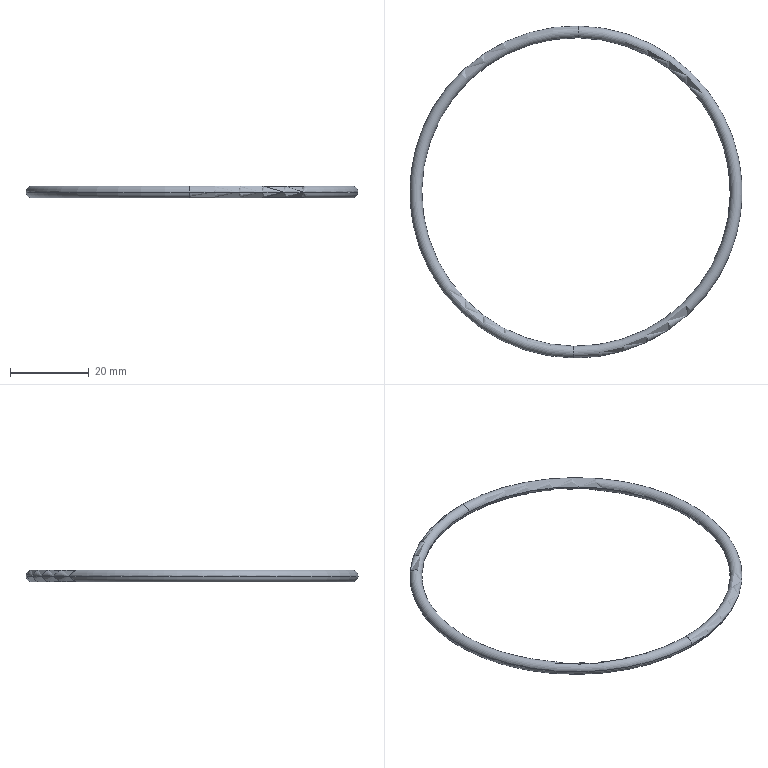Part | SolidWorks | features BaseBody 1 | 1 solid | 4 faces | box 84.4 x 84.4 x 3 mm | volume 1808 mm3 | torus 4
STEP:
#1=CARTESIAN_POINT('',(-43.838,-7.908,87.25));
#2=VERTEX_POINT('',#1);
#3=CARTESIAN_POINT('',(-43.882,-10.908,87.25));
#4=VERTEX_POINT('',#3);
#5=CARTESIAN_POINT('',(-43.86,-9.408,87.25));
#6=DIRECTION('',(-0.9999,0.01482,0.));
#7=DIRECTION('',(-0.01482,-0.9999,0.));
#8=AXIS2_PLACEMENT_3D('',#5,#6,#7);
#9=CIRCLE('',#8,1.5);
#10=EDGE_CURVE('',#2,#4,#9,.T.);
#11=ORIENTED_EDGE('',*,*,#10,.F.);
#12=CARTESIAN_POINT('',(-45.088,-92.299,87.25));
#13=VERTEX_POINT('',#12);
#14=CARTESIAN_POINT('',(-44.463,-50.104,87.25));
#15=DIRECTION('',(0.,0.,-1.));
#16=DIRECTION('',(-1.,0.,0.));
#17=AXIS2_PLACEMENT_3D('',#14,#15,#16);
#18=CIRCLE('',#17,42.2);
#19=EDGE_CURVE('',#2,#13,#18,.T.);
#20=ORIENTED_EDGE('',*,*,#19,.T.);
#21=CARTESIAN_POINT('',(-45.044,-89.299,87.25));
#22=VERTEX_POINT('',#21);
#23=CARTESIAN_POINT('',(-45.066,-90.799,87.25));
#24=DIRECTION('',(0.9999,-0.01482,0.));
#25=DIRECTION('',(0.01482,0.9999,0.));
#26=AXIS2_PLACEMENT_3D('',#23,#24,#25);
#27=CIRCLE('',#26,1.5);
#28=EDGE_CURVE('',#13,#22,#27,.T.);
#29=ORIENTED_EDGE('',*,*,#28,.T.);
#30=CARTESIAN_POINT('',(-44.463,-50.104,87.25));
#31=DIRECTION('',(0.,0.,-1.));
#32=DIRECTION('',(-1.,0.,0.));
#33=AXIS2_PLACEMENT_3D('',#30,#31,#32);
#34=CIRCLE('',#33,39.2);
#35=EDGE_CURVE('',#4,#22,#34,.T.);
#36=ORIENTED_EDGE('',*,*,#35,.F.);
#37=EDGE_LOOP('',(#11,#20,#29,#36));
#38=FACE_OUTER_BOUND('',#37,.T.);
#39=CARTESIAN_POINT('',(-44.463,-50.104,87.25));
#40=DIRECTION('',(0.,0.,-1.));
#41=DIRECTION('',(-0.01482,-0.9999,0.));
#42=AXIS2_PLACEMENT_3D('',#39,#40,#41);
#43=TOROIDAL_SURFACE('',#42,40.7,1.5);
#44=ADVANCED_FACE('',(#38),#43,.T.);
#45=ORIENTED_EDGE('',*,*,#28,.F.);
#46=CARTESIAN_POINT('',(-44.463,-50.104,87.25));
#47=DIRECTION('',(0.,0.,-1.));
#48=DIRECTION('',(-1.,0.,0.));
#49=AXIS2_PLACEMENT_3D('',#46,#47,#48);
#50=CIRCLE('',#49,42.2);
#51=EDGE_CURVE('',#13,#2,#50,.T.);
#52=ORIENTED_EDGE('',*,*,#51,.T.);
#53=ORIENTED_EDGE('',*,*,#10,.T.);
#54=CARTESIAN_POINT('',(-44.463,-50.104,87.25));
#55=DIRECTION('',(0.,0.,-1.));
#56=DIRECTION('',(-1.,0.,0.));
#57=AXIS2_PLACEMENT_3D('',#54,#55,#56);
#58=CIRCLE('',#57,39.2);
#59=EDGE_CURVE('',#22,#4,#58,.T.);
#60=ORIENTED_EDGE('',*,*,#59,.F.);
#61=EDGE_LOOP('',(#45,#52,#53,#60));
#62=FACE_OUTER_BOUND('',#61,.T.);
#63=CARTESIAN_POINT('',(-44.463,-50.104,87.25));
#64=DIRECTION('',(0.,0.,-1.));
#65=DIRECTION('',(-0.01482,-0.9999,0.));
#66=AXIS2_PLACEMENT_3D('',#63,#64,#65);
#67=TOROIDAL_SURFACE('',#66,40.7,1.5);
#68=ADVANCED_FACE('',(#62),#67,.T.);
#69=ORIENTED_EDGE('',*,*,#51,.F.);
#70=CARTESIAN_POINT('',(-45.066,-90.799,87.25));
#71=DIRECTION('',(0.9999,-0.01482,0.));
#72=DIRECTION('',(0.01482,0.9999,0.));
#73=AXIS2_PLACEMENT_3D('',#70,#71,#72);
#74=CIRCLE('',#73,1.5);
#75=EDGE_CURVE('',#22,#13,#74,.T.);
#76=ORIENTED_EDGE('',*,*,#75,.F.);
#77=ORIENTED_EDGE('',*,*,#59,.T.);
#78=CARTESIAN_POINT('',(-43.86,-9.408,87.25));
#79=DIRECTION('',(-0.9999,0.01482,0.));
#80=DIRECTION('',(-0.01482,-0.9999,0.));
#81=AXIS2_PLACEMENT_3D('',#78,#79,#80);
#82=CIRCLE('',#81,1.5);
#83=EDGE_CURVE('',#4,#2,#82,.T.);
#84=ORIENTED_EDGE('',*,*,#83,.T.);
#85=EDGE_LOOP('',(#69,#76,#77,#84));
#86=FACE_OUTER_BOUND('',#85,.T.);
#87=CARTESIAN_POINT('',(-44.463,-50.104,87.25));
#88=DIRECTION('',(0.,0.,-1.));
#89=DIRECTION('',(-0.01482,-0.9999,0.));
#90=AXIS2_PLACEMENT_3D('',#87,#88,#89);
#91=TOROIDAL_SURFACE('',#90,40.7,1.5);
#92=ADVANCED_FACE('',(#86),#91,.T.);
#93=ORIENTED_EDGE('',*,*,#19,.F.);
#94=ORIENTED_EDGE('',*,*,#83,.F.);
#95=ORIENTED_EDGE('',*,*,#35,.T.);
#96=ORIENTED_EDGE('',*,*,#75,.T.);
#97=EDGE_LOOP('',(#93,#94,#95,#96));
#98=FACE_OUTER_BOUND('',#97,.T.);
#99=CARTESIAN_POINT('',(-44.463,-50.104,87.25));
#100=DIRECTION('',(0.,0.,-1.));
#101=DIRECTION('',(-0.01482,-0.9999,0.));
#102=AXIS2_PLACEMENT_3D('',#99,#100,#101);
#103=TOROIDAL_SURFACE('',#102,40.7,1.5);
#104=ADVANCED_FACE('',(#98),#103,.T.);
#105=CLOSED_SHELL('',(#44,#68,#92,#104));
#106=MANIFOLD_SOLID_BREP('',#105);
#107=CARTESIAN_POINT('',(0.,0.,0.));
#108=DIRECTION('',(0.,0.,1.));
#109=DIRECTION('',(1.,0.,0.));
#110=AXIS2_PLACEMENT_3D('',#107,#108,#109);
#111=(LENGTH_UNIT()NAMED_UNIT(*)SI_UNIT(.MILLI.,.METRE.));
#112=UNCERTAINTY_MEASURE_WITH_UNIT(LENGTH_MEASURE(0.00001),#111,'','');
#113=(NAMED_UNIT(*)PLANE_ANGLE_UNIT()SI_UNIT($,.RADIAN.));
#114=(NAMED_UNIT(*)SI_UNIT($,.STERADIAN.)SOLID_ANGLE_UNIT());
#115=(GEOMETRIC_REPRESENTATION_CONTEXT(3)GLOBAL_UNCERTAINTY_ASSIGNED_CONTEXT((#112))GLOBAL_UNIT_ASSIGNED_CONTEXT((#111,#113,#114))REPRESENTATION_CONTEXT('',''));
#116=ADVANCED_BREP_SHAPE_REPRESENTATION('',(#106,#110),#115);